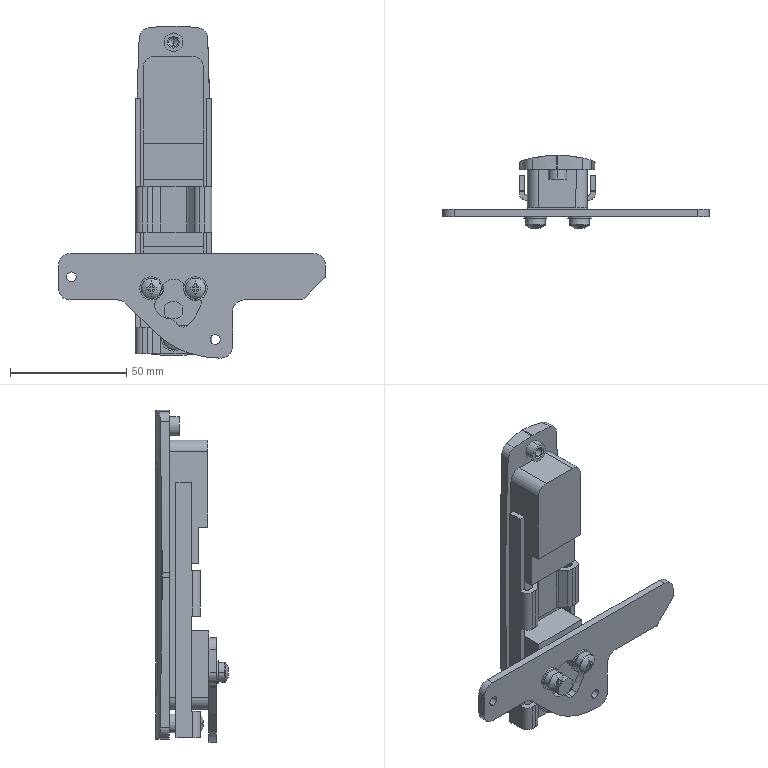Part | SolidWorks | features BaseBody 1 | 1 solid | 259 faces | box 115 x 31.4 x 143 mm | volume 78336 mm3 | cylinder 125 | plane 112 | cone 10 | spline 6 | torus 6 | commonest cylinder face diameters 10 x19 2 x16 8.136 x15 6.6 x12 1 x6 8 x6